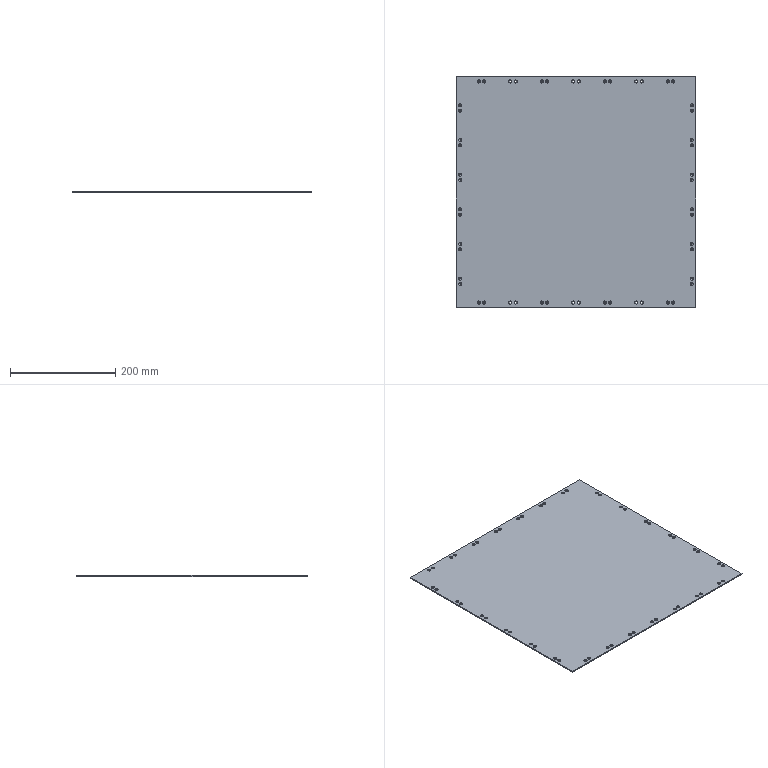Part | STEP file | Chassis cover | 1 solid | 162 faces | box 456 x 438 x 2 mm | volume 397913 mm3 | cone 104 | cylinder 52 | plane 6 | commonest cylinder face diameters 3.2 x52